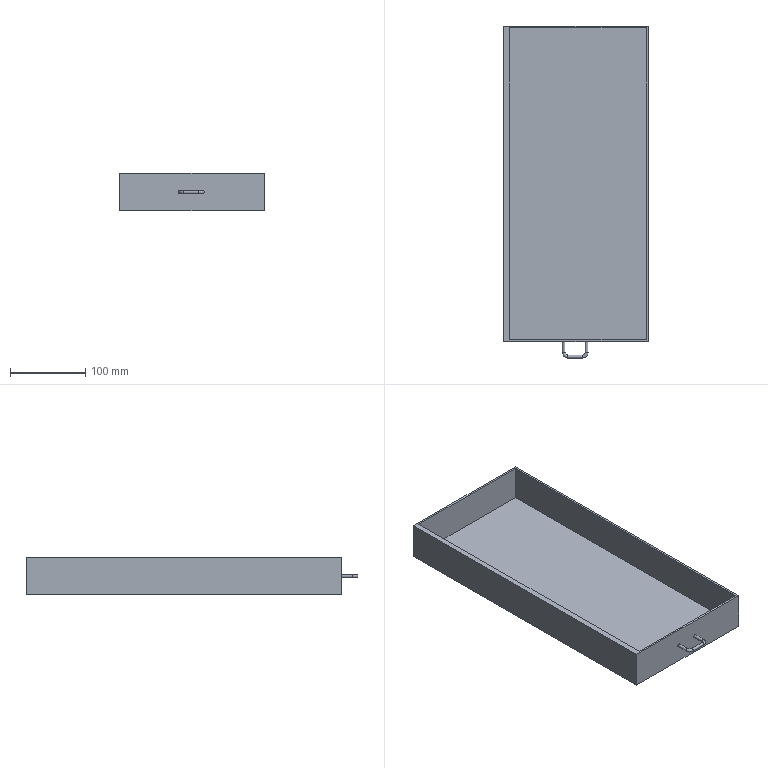Part | NX | features solid 2 | 1 solid | 16 faces | box 192 x 442 x 50 mm | volume 445151 mm3 | plane 11 | cylinder 3 | torus 2 | commonest cylinder face diameters 4 x3
STEP:
#1=CARTESIAN_POINT('',(-147.,-375.,-383.));
#2=VERTEX_POINT('',#1);
#3=CARTESIAN_POINT('',(-147.,-375.,-385.));
#4=DIRECTION('',(0.,-1.,0.));
#5=DIRECTION('',(0.,0.,1.));
#6=AXIS2_PLACEMENT_3D('',#3,#4,#5);
#7=CIRCLE('',#6,2.);
#8=EDGE_CURVE('',#2,#2,#7,.T.);
#9=ORIENTED_EDGE('',*,*,#8,.F.);
#10=EDGE_LOOP('',(#9));
#11=FACE_BOUND('',#10,.T.);
#12=CARTESIAN_POINT('',(-65.,-375.,-410.));
#13=VERTEX_POINT('',#12);
#14=CARTESIAN_POINT('',(-257.,-375.,-410.));
#15=VERTEX_POINT('',#14);
#16=CARTESIAN_POINT('',(-52.,-375.,-410.));
#17=DIRECTION('',(-1.,0.,0.));
#18=VECTOR('',#17,1000.);
#19=LINE('',#16,#18);
#20=EDGE_CURVE('',#13,#15,#19,.T.);
#21=ORIENTED_EDGE('',*,*,#20,.F.);
#22=CARTESIAN_POINT('',(-65.,-375.,-360.));
#23=VERTEX_POINT('',#22);
#24=CARTESIAN_POINT('',(-65.,-375.,-300.));
#25=DIRECTION('',(0.,0.,-1.));
#26=VECTOR('',#25,1000.);
#27=LINE('',#24,#26);
#28=EDGE_CURVE('',#23,#13,#27,.T.);
#29=ORIENTED_EDGE('',*,*,#28,.F.);
#30=CARTESIAN_POINT('',(-257.,-375.,-360.));
#31=VERTEX_POINT('',#30);
#32=CARTESIAN_POINT('',(-52.,-375.,-360.));
#33=DIRECTION('',(-1.,0.,0.));
#34=VECTOR('',#33,1000.);
#35=LINE('',#32,#34);
#36=EDGE_CURVE('',#23,#31,#35,.T.);
#37=ORIENTED_EDGE('',*,*,#36,.T.);
#38=CARTESIAN_POINT('',(-257.,-375.,-270.));
#39=DIRECTION('',(0.,0.,-1.));
#40=VECTOR('',#39,1000.);
#41=LINE('',#38,#40);
#42=EDGE_CURVE('',#31,#15,#41,.T.);
#43=ORIENTED_EDGE('',*,*,#42,.T.);
#44=EDGE_LOOP('',(#21,#29,#37,#43));
#45=FACE_BOUND('',#44,.T.);
#46=CARTESIAN_POINT('',(-177.,-375.,-383.));
#47=VERTEX_POINT('',#46);
#48=CARTESIAN_POINT('',(-177.,-375.,-385.));
#49=DIRECTION('',(0.,-1.,0.));
#50=DIRECTION('',(0.,0.,1.));
#51=AXIS2_PLACEMENT_3D('',#48,#49,#50);
#52=CIRCLE('',#51,2.);
#53=EDGE_CURVE('',#47,#47,#52,.T.);
#54=ORIENTED_EDGE('',*,*,#53,.F.);
#55=EDGE_LOOP('',(#54));
#56=FACE_BOUND('',#55,.T.);
#57=CARTESIAN_POINT('',(-52.,-375.,-360.));
#58=DIRECTION('',(0.,-1.,0.));
#59=DIRECTION('',(0.,0.,1.));
#60=AXIS2_PLACEMENT_3D('',#57,#58,#59);
#61=PLANE('',#60);
#62=ADVANCED_FACE('',(#11,#45,#56),#61,.T.);
#63=CARTESIAN_POINT('',(-249.5,-372.5,-407.5));
#64=VERTEX_POINT('',#63);
#65=CARTESIAN_POINT('',(-249.5,42.5,-407.5));
#66=VERTEX_POINT('',#65);
#67=CARTESIAN_POINT('',(-249.5,-252.5,-407.5));
#68=DIRECTION('',(0.,1.,0.));
#69=VECTOR('',#68,1000.);
#70=LINE('',#67,#69);
#71=EDGE_CURVE('',#64,#66,#70,.T.);
#72=ORIENTED_EDGE('',*,*,#71,.F.);
#73=CARTESIAN_POINT('',(-67.5,-372.5,-407.5));
#74=VERTEX_POINT('',#73);
#75=CARTESIAN_POINT('',(-202.,-372.5,-407.5));
#76=DIRECTION('',(-1.,0.,0.));
#77=VECTOR('',#76,1000.);
#78=LINE('',#75,#77);
#79=EDGE_CURVE('',#74,#64,#78,.T.);
#80=ORIENTED_EDGE('',*,*,#79,.F.);
#81=CARTESIAN_POINT('',(-67.5,42.5,-407.5));
#82=VERTEX_POINT('',#81);
#83=CARTESIAN_POINT('',(-67.5,-252.5,-407.5));
#84=DIRECTION('',(0.,-1.,0.));
#85=VECTOR('',#84,1000.);
#86=LINE('',#83,#85);
#87=EDGE_CURVE('',#82,#74,#86,.T.);
#88=ORIENTED_EDGE('',*,*,#87,.F.);
#89=CARTESIAN_POINT('',(-199.5,42.5,-407.5));
#90=DIRECTION('',(1.,0.,0.));
#91=VECTOR('',#90,1000.);
#92=LINE('',#89,#91);
#93=EDGE_CURVE('',#66,#82,#92,.T.);
#94=ORIENTED_EDGE('',*,*,#93,.F.);
#95=EDGE_LOOP('',(#72,#80,#88,#94));
#96=FACE_BOUND('',#95,.T.);
#97=CARTESIAN_POINT('',(-199.5,-252.5,-407.5));
#98=DIRECTION('',(0.,0.,-1.));
#99=DIRECTION('',(1.,0.,0.));
#100=AXIS2_PLACEMENT_3D('',#97,#98,#99);
#101=PLANE('',#100);
#102=ADVANCED_FACE('',(#96),#101,.F.);
#103=CARTESIAN_POINT('',(-257.,45.,-410.));
#104=VERTEX_POINT('',#103);
#105=CARTESIAN_POINT('',(-65.,45.,-410.));
#106=VERTEX_POINT('',#105);
#107=CARTESIAN_POINT('',(-199.5,45.,-410.));
#108=DIRECTION('',(1.,0.,0.));
#109=VECTOR('',#108,1000.);
#110=LINE('',#107,#109);
#111=EDGE_CURVE('',#104,#106,#110,.T.);
#112=ORIENTED_EDGE('',*,*,#111,.T.);
#113=CARTESIAN_POINT('',(-65.,-182.5,-410.));
#114=DIRECTION('',(0.,-1.,0.));
#115=VECTOR('',#114,1000.);
#116=LINE('',#113,#115);
#117=EDGE_CURVE('',#106,#13,#116,.T.);
#118=ORIENTED_EDGE('',*,*,#117,.T.);
#119=ORIENTED_EDGE('',*,*,#20,.T.);
#120=CARTESIAN_POINT('',(-257.,156.,-410.));
#121=DIRECTION('',(0.,1.,0.));
#122=VECTOR('',#121,1000.);
#123=LINE('',#120,#122);
#124=EDGE_CURVE('',#15,#104,#123,.T.);
#125=ORIENTED_EDGE('',*,*,#124,.T.);
#126=EDGE_LOOP('',(#112,#118,#119,#125));
#127=FACE_BOUND('',#126,.T.);
#128=CARTESIAN_POINT('',(-199.5,-182.5,-410.));
#129=DIRECTION('',(0.,0.,-1.));
#130=DIRECTION('',(1.,0.,0.));
#131=AXIS2_PLACEMENT_3D('',#128,#129,#130);
#132=PLANE('',#131);
#133=ADVANCED_FACE('',(#127),#132,.T.);
#134=CARTESIAN_POINT('',(-249.5,-372.5,-360.));
#135=VERTEX_POINT('',#134);
#136=CARTESIAN_POINT('',(-249.5,-372.5,-360.));
#137=DIRECTION('',(0.,0.,-1.));
#138=VECTOR('',#137,1000.);
#139=LINE('',#136,#138);
#140=EDGE_CURVE('',#135,#64,#139,.T.);
#141=ORIENTED_EDGE('',*,*,#140,.F.);
#142=CARTESIAN_POINT('',(-67.5,-372.5,-360.));
#143=VERTEX_POINT('',#142);
#144=CARTESIAN_POINT('',(-202.,-372.5,-360.));
#145=DIRECTION('',(1.,0.,0.));
#146=VECTOR('',#145,1000.);
#147=LINE('',#144,#146);
#148=EDGE_CURVE('',#135,#143,#147,.T.);
#149=ORIENTED_EDGE('',*,*,#148,.T.);
#150=CARTESIAN_POINT('',(-67.5,-372.5,-300.));
#151=DIRECTION('',(0.,0.,-1.));
#152=VECTOR('',#151,1000.);
#153=LINE('',#150,#152);
#154=EDGE_CURVE('',#143,#74,#153,.T.);
#155=ORIENTED_EDGE('',*,*,#154,.T.);
#156=ORIENTED_EDGE('',*,*,#79,.T.);
#157=EDGE_LOOP('',(#141,#149,#155,#156));
#158=FACE_BOUND('',#157,.T.);
#159=CARTESIAN_POINT('',(-202.,-372.5,-360.));
#160=DIRECTION('',(0.,1.,0.));
#161=DIRECTION('',(0.,0.,-1.));
#162=AXIS2_PLACEMENT_3D('',#159,#160,#161);
#163=PLANE('',#162);
#164=ADVANCED_FACE('',(#158),#163,.T.);
#165=ORIENTED_EDGE('',*,*,#124,.F.);
#166=ORIENTED_EDGE('',*,*,#42,.F.);
#167=CARTESIAN_POINT('',(-257.,45.,-360.));
#168=VERTEX_POINT('',#167);
#169=CARTESIAN_POINT('',(-257.,156.,-360.));
#170=DIRECTION('',(0.,1.,0.));
#171=VECTOR('',#170,1000.);
#172=LINE('',#169,#171);
#173=EDGE_CURVE('',#31,#168,#172,.T.);
#174=ORIENTED_EDGE('',*,*,#173,.T.);
#175=CARTESIAN_POINT('',(-257.,45.,-360.));
#176=DIRECTION('',(0.,0.,-1.));
#177=VECTOR('',#176,1000.);
#178=LINE('',#175,#177);
#179=EDGE_CURVE('',#168,#104,#178,.T.);
#180=ORIENTED_EDGE('',*,*,#179,.T.);
#181=EDGE_LOOP('',(#165,#166,#174,#180));
#182=FACE_BOUND('',#181,.T.);
#183=CARTESIAN_POINT('',(-257.,156.,-270.));
#184=DIRECTION('',(1.,0.,0.));
#185=DIRECTION('',(0.,0.,1.));
#186=AXIS2_PLACEMENT_3D('',#183,#184,#185);
#187=PLANE('',#186);
#188=ADVANCED_FACE('',(#182),#187,.F.);
#189=ORIENTED_EDGE('',*,*,#117,.F.);
#190=CARTESIAN_POINT('',(-65.,45.,-360.));
#191=VERTEX_POINT('',#190);
#192=CARTESIAN_POINT('',(-65.,45.,-300.));
#193=DIRECTION('',(0.,0.,-1.));
#194=VECTOR('',#193,1000.);
#195=LINE('',#192,#194);
#196=EDGE_CURVE('',#191,#106,#195,.T.);
#197=ORIENTED_EDGE('',*,*,#196,.F.);
#198=CARTESIAN_POINT('',(-65.,-372.5,-360.));
#199=DIRECTION('',(0.,-1.,0.));
#200=VECTOR('',#199,1000.);
#201=LINE('',#198,#200);
#202=EDGE_CURVE('',#191,#23,#201,.T.);
#203=ORIENTED_EDGE('',*,*,#202,.T.);
#204=ORIENTED_EDGE('',*,*,#28,.T.);
#205=EDGE_LOOP('',(#189,#197,#203,#204));
#206=FACE_BOUND('',#205,.T.);
#207=CARTESIAN_POINT('',(-65.,80.624,-300.));
#208=DIRECTION('',(-1.,0.,0.));
#209=DIRECTION('',(0.,0.,-1.));
#210=AXIS2_PLACEMENT_3D('',#207,#208,#209);
#211=PLANE('',#210);
#212=ADVANCED_FACE('',(#206),#211,.F.);
#213=ORIENTED_EDGE('',*,*,#148,.F.);
#214=CARTESIAN_POINT('',(-249.5,42.5,-360.));
#215=VERTEX_POINT('',#214);
#216=CARTESIAN_POINT('',(-249.5,-372.5,-360.));
#217=DIRECTION('',(0.,-1.,0.));
#218=VECTOR('',#217,1000.);
#219=LINE('',#216,#218);
#220=EDGE_CURVE('',#215,#135,#219,.T.);
#221=ORIENTED_EDGE('',*,*,#220,.F.);
#222=CARTESIAN_POINT('',(-67.5,42.5,-360.));
#223=VERTEX_POINT('',#222);
#224=CARTESIAN_POINT('',(-202.,42.5,-360.));
#225=DIRECTION('',(-1.,0.,0.));
#226=VECTOR('',#225,1000.);
#227=LINE('',#224,#226);
#228=EDGE_CURVE('',#223,#215,#227,.T.);
#229=ORIENTED_EDGE('',*,*,#228,.F.);
#230=CARTESIAN_POINT('',(-67.5,80.624,-360.));
#231=DIRECTION('',(0.,1.,0.));
#232=VECTOR('',#231,1000.);
#233=LINE('',#230,#232);
#234=EDGE_CURVE('',#143,#223,#233,.T.);
#235=ORIENTED_EDGE('',*,*,#234,.F.);
#236=EDGE_LOOP('',(#213,#221,#229,#235));
#237=FACE_BOUND('',#236,.T.);
#238=ORIENTED_EDGE('',*,*,#173,.F.);
#239=ORIENTED_EDGE('',*,*,#36,.F.);
#240=ORIENTED_EDGE('',*,*,#202,.F.);
#241=CARTESIAN_POINT('',(-202.,45.,-360.));
#242=DIRECTION('',(1.,0.,0.));
#243=VECTOR('',#242,1000.);
#244=LINE('',#241,#243);
#245=EDGE_CURVE('',#168,#191,#244,.T.);
#246=ORIENTED_EDGE('',*,*,#245,.F.);
#247=EDGE_LOOP('',(#238,#239,#240,#246));
#248=FACE_BOUND('',#247,.T.);
#249=CARTESIAN_POINT('',(-202.,-372.5,-360.));
#250=DIRECTION('',(0.,0.,-1.));
#251=DIRECTION('',(1.,0.,0.));
#252=AXIS2_PLACEMENT_3D('',#249,#250,#251);
#253=PLANE('',#252);
#254=ADVANCED_FACE('',(#237,#248),#253,.F.);
#255=CARTESIAN_POINT('',(-249.5,42.5,-360.));
#256=DIRECTION('',(0.,0.,-1.));
#257=VECTOR('',#256,1000.);
#258=LINE('',#255,#257);
#259=EDGE_CURVE('',#215,#66,#258,.T.);
#260=ORIENTED_EDGE('',*,*,#259,.T.);
#261=ORIENTED_EDGE('',*,*,#93,.T.);
#262=CARTESIAN_POINT('',(-67.5,42.5,-300.));
#263=DIRECTION('',(0.,0.,-1.));
#264=VECTOR('',#263,1000.);
#265=LINE('',#262,#264);
#266=EDGE_CURVE('',#223,#82,#265,.T.);
#267=ORIENTED_EDGE('',*,*,#266,.F.);
#268=ORIENTED_EDGE('',*,*,#228,.T.);
#269=EDGE_LOOP('',(#260,#261,#267,#268));
#270=FACE_BOUND('',#269,.T.);
#271=CARTESIAN_POINT('',(-52.,42.5,-360.));
#272=DIRECTION('',(0.,-1.,0.));
#273=DIRECTION('',(0.,0.,1.));
#274=AXIS2_PLACEMENT_3D('',#271,#272,#273);
#275=PLANE('',#274);
#276=ADVANCED_FACE('',(#270),#275,.T.);
#277=ORIENTED_EDGE('',*,*,#111,.F.);
#278=ORIENTED_EDGE('',*,*,#179,.F.);
#279=ORIENTED_EDGE('',*,*,#245,.T.);
#280=ORIENTED_EDGE('',*,*,#196,.T.);
#281=EDGE_LOOP('',(#277,#278,#279,#280));
#282=FACE_BOUND('',#281,.T.);
#283=CARTESIAN_POINT('',(-202.,45.,-360.));
#284=DIRECTION('',(0.,1.,0.));
#285=DIRECTION('',(0.,0.,-1.));
#286=AXIS2_PLACEMENT_3D('',#283,#284,#285);
#287=PLANE('',#286);
#288=ADVANCED_FACE('',(#282),#287,.T.);
#289=ORIENTED_EDGE('',*,*,#87,.T.);
#290=ORIENTED_EDGE('',*,*,#154,.F.);
#291=ORIENTED_EDGE('',*,*,#234,.T.);
#292=ORIENTED_EDGE('',*,*,#266,.T.);
#293=EDGE_LOOP('',(#289,#290,#291,#292));
#294=FACE_BOUND('',#293,.T.);
#295=CARTESIAN_POINT('',(-67.5,10.624,-300.));
#296=DIRECTION('',(-1.,0.,0.));
#297=DIRECTION('',(0.,0.,-1.));
#298=AXIS2_PLACEMENT_3D('',#295,#296,#297);
#299=PLANE('',#298);
#300=ADVANCED_FACE('',(#294),#299,.T.);
#301=ORIENTED_EDGE('',*,*,#71,.T.);
#302=ORIENTED_EDGE('',*,*,#259,.F.);
#303=ORIENTED_EDGE('',*,*,#220,.T.);
#304=ORIENTED_EDGE('',*,*,#140,.T.);
#305=EDGE_LOOP('',(#301,#302,#303,#304));
#306=FACE_BOUND('',#305,.T.);
#307=CARTESIAN_POINT('',(-249.5,-252.5,-360.));
#308=DIRECTION('',(1.,0.,0.));
#309=DIRECTION('',(0.,0.,1.));
#310=AXIS2_PLACEMENT_3D('',#307,#308,#309);
#311=PLANE('',#310);
#312=ADVANCED_FACE('',(#306),#311,.T.);
#313=CARTESIAN_POINT('',(-147.,-390.,-383.));
#314=VERTEX_POINT('',#313);
#315=CARTESIAN_POINT('',(-147.,-390.,-385.));
#316=DIRECTION('',(0.,1.,0.));
#317=DIRECTION('',(0.,0.,1.));
#318=AXIS2_PLACEMENT_3D('',#315,#316,#317);
#319=CIRCLE('',#318,2.);
#320=EDGE_CURVE('',#314,#314,#319,.T.);
#321=ORIENTED_EDGE('',*,*,#320,.T.);
#322=EDGE_LOOP('',(#321));
#323=FACE_BOUND('',#322,.T.);
#324=ORIENTED_EDGE('',*,*,#8,.T.);
#325=EDGE_LOOP('',(#324));
#326=FACE_BOUND('',#325,.T.);
#327=CARTESIAN_POINT('',(-147.,-390.,-385.));
#328=DIRECTION('',(0.,1.,0.));
#329=DIRECTION('',(0.,0.,-1.));
#330=AXIS2_PLACEMENT_3D('',#327,#328,#329);
#331=CYLINDRICAL_SURFACE('',#330,2.);
#332=ADVANCED_FACE('',(#323,#326),#331,.T.);
#333=CARTESIAN_POINT('',(-152.,-395.,-383.));
#334=VERTEX_POINT('',#333);
#335=CARTESIAN_POINT('',(-152.,-395.,-385.));
#336=DIRECTION('',(1.,0.,0.));
#337=DIRECTION('',(0.,0.,1.));
#338=AXIS2_PLACEMENT_3D('',#335,#336,#337);
#339=CIRCLE('',#338,2.);
#340=EDGE_CURVE('',#334,#334,#339,.T.);
#341=ORIENTED_EDGE('',*,*,#340,.T.);
#342=EDGE_LOOP('',(#341));
#343=FACE_BOUND('',#342,.T.);
#344=ORIENTED_EDGE('',*,*,#320,.F.);
#345=EDGE_LOOP('',(#344));
#346=FACE_BOUND('',#345,.T.);
#347=CARTESIAN_POINT('',(-152.,-390.,-385.));
#348=DIRECTION('',(0.,0.,1.));
#349=DIRECTION('',(-1.,0.,0.));
#350=AXIS2_PLACEMENT_3D('',#347,#348,#349);
#351=TOROIDAL_SURFACE('',#350,5.,2.);
#352=ADVANCED_FACE('',(#343,#346),#351,.T.);
#353=CARTESIAN_POINT('',(-172.,-395.,-383.));
#354=VERTEX_POINT('',#353);
#355=CARTESIAN_POINT('',(-172.,-395.,-385.));
#356=DIRECTION('',(1.,0.,0.));
#357=DIRECTION('',(0.,0.,1.));
#358=AXIS2_PLACEMENT_3D('',#355,#356,#357);
#359=CIRCLE('',#358,2.);
#360=EDGE_CURVE('',#354,#354,#359,.T.);
#361=ORIENTED_EDGE('',*,*,#360,.T.);
#362=EDGE_LOOP('',(#361));
#363=FACE_BOUND('',#362,.T.);
#364=ORIENTED_EDGE('',*,*,#340,.F.);
#365=EDGE_LOOP('',(#364));
#366=FACE_BOUND('',#365,.T.);
#367=CARTESIAN_POINT('',(-172.,-395.,-385.));
#368=DIRECTION('',(1.,0.,0.));
#369=DIRECTION('',(0.,0.,1.));
#370=AXIS2_PLACEMENT_3D('',#367,#368,#369);
#371=CYLINDRICAL_SURFACE('',#370,2.);
#372=ADVANCED_FACE('',(#363,#366),#371,.T.);
#373=CARTESIAN_POINT('',(-177.,-390.,-383.));
#374=VERTEX_POINT('',#373);
#375=CARTESIAN_POINT('',(-177.,-390.,-385.));
#376=DIRECTION('',(0.,-1.,0.));
#377=DIRECTION('',(0.,0.,1.));
#378=AXIS2_PLACEMENT_3D('',#375,#376,#377);
#379=CIRCLE('',#378,2.);
#380=EDGE_CURVE('',#374,#374,#379,.T.);
#381=ORIENTED_EDGE('',*,*,#380,.T.);
#382=EDGE_LOOP('',(#381));
#383=FACE_BOUND('',#382,.T.);
#384=ORIENTED_EDGE('',*,*,#360,.F.);
#385=EDGE_LOOP('',(#384));
#386=FACE_BOUND('',#385,.T.);
#387=CARTESIAN_POINT('',(-172.,-390.,-385.));
#388=DIRECTION('',(0.,0.,1.));
#389=DIRECTION('',(-1.,0.,0.));
#390=AXIS2_PLACEMENT_3D('',#387,#388,#389);
#391=TOROIDAL_SURFACE('',#390,5.,2.);
#392=ADVANCED_FACE('',(#383,#386),#391,.T.);
#393=ORIENTED_EDGE('',*,*,#380,.F.);
#394=EDGE_LOOP('',(#393));
#395=FACE_BOUND('',#394,.T.);
#396=ORIENTED_EDGE('',*,*,#53,.T.);
#397=EDGE_LOOP('',(#396));
#398=FACE_BOUND('',#397,.T.);
#399=CARTESIAN_POINT('',(-177.,-390.,-385.));
#400=DIRECTION('',(0.,1.,0.));
#401=DIRECTION('',(0.,0.,-1.));
#402=AXIS2_PLACEMENT_3D('',#399,#400,#401);
#403=CYLINDRICAL_SURFACE('',#402,2.);
#404=ADVANCED_FACE('',(#395,#398),#403,.T.);
#405=CLOSED_SHELL('',(#62,#102,#133,#164,#188,#212,#254,#276,#288,#300,#312,#332,#352,#372,#392,#404));
#406=MANIFOLD_SOLID_BREP('',#405);
#407=(LENGTH_UNIT()NAMED_UNIT(*)SI_UNIT(.MILLI.,.METRE.));
#408=UNCERTAINTY_MEASURE_WITH_UNIT(LENGTH_MEASURE(0.00001),#407,'','');
#409=(NAMED_UNIT(*)PLANE_ANGLE_UNIT()SI_UNIT($,.RADIAN.));
#410=(NAMED_UNIT(*)SI_UNIT($,.STERADIAN.)SOLID_ANGLE_UNIT());
#411=(GEOMETRIC_REPRESENTATION_CONTEXT(3)GLOBAL_UNCERTAINTY_ASSIGNED_CONTEXT((#408))GLOBAL_UNIT_ASSIGNED_CONTEXT((#407,#409,#410))REPRESENTATION_CONTEXT('',''));
#412=ADVANCED_BREP_SHAPE_REPRESENTATION('',(#406),#411);